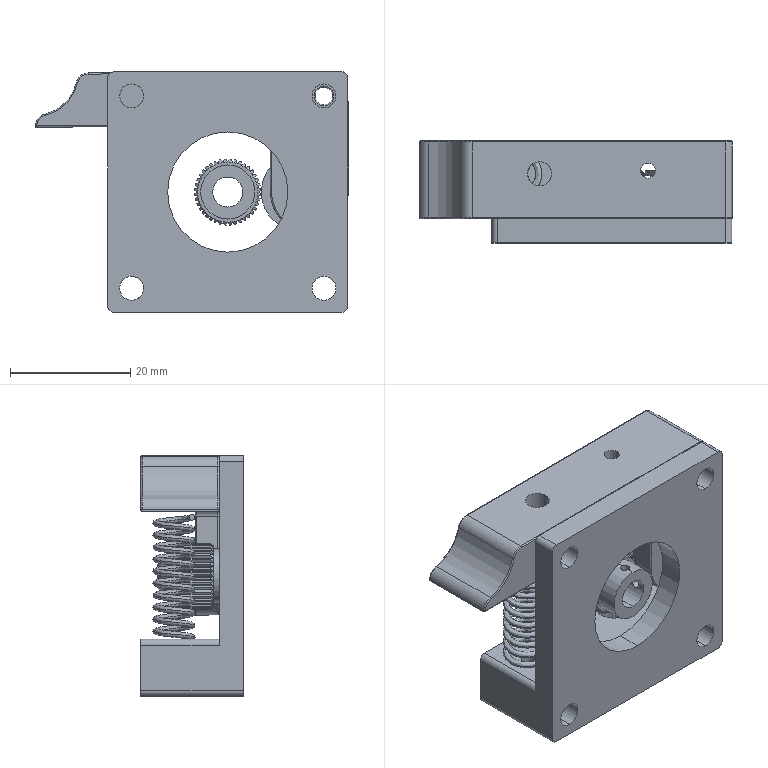Part | SolidWorks | 6 solids | 344 faces | box 52.047 x 17 x 40.013 mm | volume 16596 mm3 | plane 119 | cylinder 107 | cone 84 | torus 30 | spline 2 | sphere 2 | commonest cylinder face diameters 11 x40 4 x19 0.4 x11 2 x9 13 x5 1.5 x4